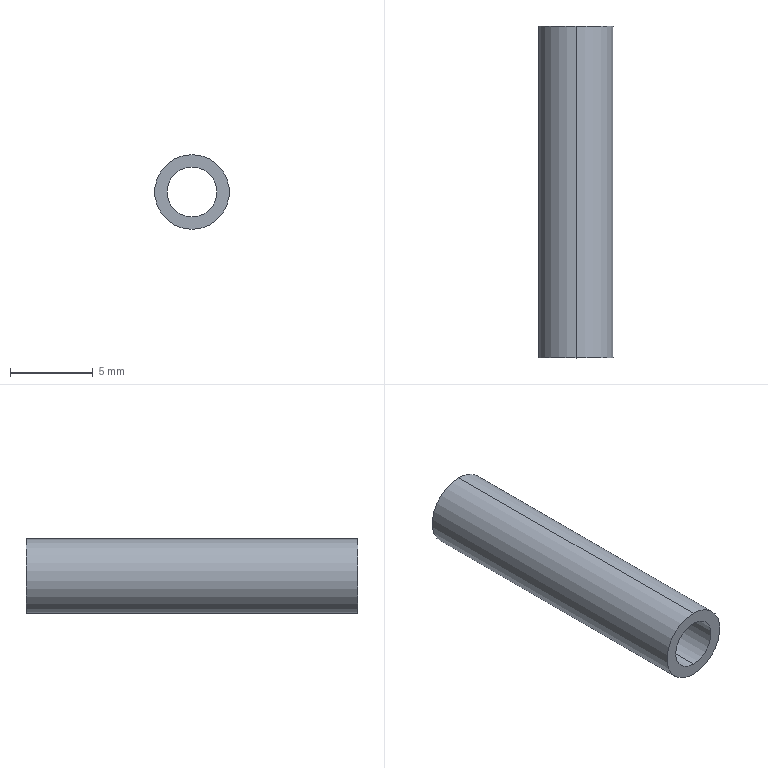Part | SolidWorks | features Extrusion 1 | 1 solid | 6 faces | box 4.5 x 20 x 4.5 mm | volume 176.715 mm3 | cylinder 4 | plane 2 | commonest cylinder face diameters 3 x2 4.5 x2
STEP:
#1=CARTESIAN_POINT('',(0.,20.,-1.5));
#2=VERTEX_POINT('',#1);
#3=CARTESIAN_POINT('',(0.,20.,1.5));
#4=VERTEX_POINT('',#3);
#5=CARTESIAN_POINT('',(0.,20.,0.));
#6=DIRECTION('',(0.,1.,0.));
#7=DIRECTION('',(0.,0.,1.));
#8=AXIS2_PLACEMENT_3D('',#5,#6,#7);
#9=CIRCLE('',#8,1.5);
#10=EDGE_CURVE('',#2,#4,#9,.T.);
#11=ORIENTED_EDGE('',*,*,#10,.T.);
#12=CARTESIAN_POINT('',(0.,0.,1.5));
#13=VERTEX_POINT('',#12);
#14=CARTESIAN_POINT('',(0.,20.,1.5));
#15=DIRECTION('',(0.,-1.,0.));
#16=VECTOR('',#15,1000.);
#17=LINE('',#14,#16);
#18=EDGE_CURVE('',#4,#13,#17,.T.);
#19=ORIENTED_EDGE('',*,*,#18,.T.);
#20=CARTESIAN_POINT('',(0.,0.,-1.5));
#21=VERTEX_POINT('',#20);
#22=CARTESIAN_POINT('',(0.,0.,0.));
#23=DIRECTION('',(0.,1.,0.));
#24=DIRECTION('',(0.,0.,1.));
#25=AXIS2_PLACEMENT_3D('',#22,#23,#24);
#26=CIRCLE('',#25,1.5);
#27=EDGE_CURVE('',#21,#13,#26,.T.);
#28=ORIENTED_EDGE('',*,*,#27,.F.);
#29=CARTESIAN_POINT('',(0.,20.,-1.5));
#30=DIRECTION('',(0.,-1.,0.));
#31=VECTOR('',#30,1000.);
#32=LINE('',#29,#31);
#33=EDGE_CURVE('',#2,#21,#32,.T.);
#34=ORIENTED_EDGE('',*,*,#33,.F.);
#35=EDGE_LOOP('',(#11,#19,#28,#34));
#36=FACE_OUTER_BOUND('',#35,.T.);
#37=CARTESIAN_POINT('',(0.,20.,0.));
#38=DIRECTION('',(0.,-1.,0.));
#39=DIRECTION('',(0.,0.,-1.));
#40=AXIS2_PLACEMENT_3D('',#37,#38,#39);
#41=CYLINDRICAL_SURFACE('',#40,1.5);
#42=ADVANCED_FACE('',(#36),#41,.F.);
#43=CARTESIAN_POINT('',(0.,20.,2.25));
#44=VERTEX_POINT('',#43);
#45=CARTESIAN_POINT('',(0.,20.,-2.25));
#46=VERTEX_POINT('',#45);
#47=CARTESIAN_POINT('',(0.,20.,0.));
#48=DIRECTION('',(0.,1.,0.));
#49=DIRECTION('',(0.,0.,1.));
#50=AXIS2_PLACEMENT_3D('',#47,#48,#49);
#51=CIRCLE('',#50,2.25);
#52=EDGE_CURVE('',#44,#46,#51,.T.);
#53=ORIENTED_EDGE('',*,*,#52,.F.);
#54=CARTESIAN_POINT('',(0.,0.,2.25));
#55=VERTEX_POINT('',#54);
#56=CARTESIAN_POINT('',(0.,20.,2.25));
#57=DIRECTION('',(0.,-1.,0.));
#58=VECTOR('',#57,1000.);
#59=LINE('',#56,#58);
#60=EDGE_CURVE('',#44,#55,#59,.T.);
#61=ORIENTED_EDGE('',*,*,#60,.T.);
#62=CARTESIAN_POINT('',(0.,0.,-2.25));
#63=VERTEX_POINT('',#62);
#64=CARTESIAN_POINT('',(0.,0.,0.));
#65=DIRECTION('',(0.,1.,0.));
#66=DIRECTION('',(0.,0.,1.));
#67=AXIS2_PLACEMENT_3D('',#64,#65,#66);
#68=CIRCLE('',#67,2.25);
#69=EDGE_CURVE('',#55,#63,#68,.T.);
#70=ORIENTED_EDGE('',*,*,#69,.T.);
#71=CARTESIAN_POINT('',(0.,20.,-2.25));
#72=DIRECTION('',(0.,-1.,0.));
#73=VECTOR('',#72,1000.);
#74=LINE('',#71,#73);
#75=EDGE_CURVE('',#46,#63,#74,.T.);
#76=ORIENTED_EDGE('',*,*,#75,.F.);
#77=EDGE_LOOP('',(#53,#61,#70,#76));
#78=FACE_OUTER_BOUND('',#77,.T.);
#79=CARTESIAN_POINT('',(0.,20.,0.));
#80=DIRECTION('',(0.,-1.,0.));
#81=DIRECTION('',(0.,0.,-1.));
#82=AXIS2_PLACEMENT_3D('',#79,#80,#81);
#83=CYLINDRICAL_SURFACE('',#82,2.25);
#84=ADVANCED_FACE('',(#78),#83,.T.);
#85=CARTESIAN_POINT('',(0.,20.,0.));
#86=DIRECTION('',(0.,1.,0.));
#87=DIRECTION('',(0.,0.,1.));
#88=AXIS2_PLACEMENT_3D('',#85,#86,#87);
#89=CIRCLE('',#88,2.25);
#90=EDGE_CURVE('',#46,#44,#89,.T.);
#91=ORIENTED_EDGE('',*,*,#90,.T.);
#92=ORIENTED_EDGE('',*,*,#52,.T.);
#93=EDGE_LOOP('',(#91,#92));
#94=FACE_OUTER_BOUND('',#93,.T.);
#95=ORIENTED_EDGE('',*,*,#10,.F.);
#96=CARTESIAN_POINT('',(0.,20.,0.));
#97=DIRECTION('',(0.,1.,0.));
#98=DIRECTION('',(0.,0.,1.));
#99=AXIS2_PLACEMENT_3D('',#96,#97,#98);
#100=CIRCLE('',#99,1.5);
#101=EDGE_CURVE('',#4,#2,#100,.T.);
#102=ORIENTED_EDGE('',*,*,#101,.F.);
#103=EDGE_LOOP('',(#95,#102));
#104=FACE_BOUND('',#103,.T.);
#105=CARTESIAN_POINT('',(0.,20.,0.));
#106=DIRECTION('',(0.,1.,0.));
#107=DIRECTION('',(0.,0.,1.));
#108=AXIS2_PLACEMENT_3D('',#105,#106,#107);
#109=PLANE('',#108);
#110=ADVANCED_FACE('',(#94,#104),#109,.T.);
#111=CARTESIAN_POINT('',(0.,0.,0.));
#112=DIRECTION('',(0.,1.,0.));
#113=DIRECTION('',(0.,0.,1.));
#114=AXIS2_PLACEMENT_3D('',#111,#112,#113);
#115=CIRCLE('',#114,2.25);
#116=EDGE_CURVE('',#63,#55,#115,.T.);
#117=ORIENTED_EDGE('',*,*,#116,.F.);
#118=ORIENTED_EDGE('',*,*,#69,.F.);
#119=EDGE_LOOP('',(#117,#118));
#120=FACE_OUTER_BOUND('',#119,.T.);
#121=ORIENTED_EDGE('',*,*,#27,.T.);
#122=CARTESIAN_POINT('',(0.,0.,0.));
#123=DIRECTION('',(0.,1.,0.));
#124=DIRECTION('',(0.,0.,1.));
#125=AXIS2_PLACEMENT_3D('',#122,#123,#124);
#126=CIRCLE('',#125,1.5);
#127=EDGE_CURVE('',#13,#21,#126,.T.);
#128=ORIENTED_EDGE('',*,*,#127,.T.);
#129=EDGE_LOOP('',(#121,#128));
#130=FACE_BOUND('',#129,.T.);
#131=CARTESIAN_POINT('',(0.,0.,0.));
#132=DIRECTION('',(0.,1.,0.));
#133=DIRECTION('',(0.,0.,1.));
#134=AXIS2_PLACEMENT_3D('',#131,#132,#133);
#135=PLANE('',#134);
#136=ADVANCED_FACE('',(#120,#130),#135,.F.);
#137=ORIENTED_EDGE('',*,*,#60,.F.);
#138=ORIENTED_EDGE('',*,*,#90,.F.);
#139=ORIENTED_EDGE('',*,*,#75,.T.);
#140=ORIENTED_EDGE('',*,*,#116,.T.);
#141=EDGE_LOOP('',(#137,#138,#139,#140));
#142=FACE_OUTER_BOUND('',#141,.T.);
#143=CARTESIAN_POINT('',(0.,20.,0.));
#144=DIRECTION('',(0.,-1.,0.));
#145=DIRECTION('',(0.,0.,-1.));
#146=AXIS2_PLACEMENT_3D('',#143,#144,#145);
#147=CYLINDRICAL_SURFACE('',#146,2.25);
#148=ADVANCED_FACE('',(#142),#147,.T.);
#149=ORIENTED_EDGE('',*,*,#18,.F.);
#150=ORIENTED_EDGE('',*,*,#101,.T.);
#151=ORIENTED_EDGE('',*,*,#33,.T.);
#152=ORIENTED_EDGE('',*,*,#127,.F.);
#153=EDGE_LOOP('',(#149,#150,#151,#152));
#154=FACE_OUTER_BOUND('',#153,.T.);
#155=CARTESIAN_POINT('',(0.,20.,0.));
#156=DIRECTION('',(0.,-1.,0.));
#157=DIRECTION('',(0.,0.,-1.));
#158=AXIS2_PLACEMENT_3D('',#155,#156,#157);
#159=CYLINDRICAL_SURFACE('',#158,1.5);
#160=ADVANCED_FACE('',(#154),#159,.F.);
#161=CLOSED_SHELL('',(#42,#84,#110,#136,#148,#160));
#162=MANIFOLD_SOLID_BREP('',#161);
#163=CARTESIAN_POINT('',(0.,0.,0.));
#164=DIRECTION('',(0.,0.,1.));
#165=DIRECTION('',(1.,0.,0.));
#166=AXIS2_PLACEMENT_3D('',#163,#164,#165);
#167=(LENGTH_UNIT()NAMED_UNIT(*)SI_UNIT(.MILLI.,.METRE.));
#168=UNCERTAINTY_MEASURE_WITH_UNIT(LENGTH_MEASURE(0.00001),#167,'','');
#169=(NAMED_UNIT(*)PLANE_ANGLE_UNIT()SI_UNIT($,.RADIAN.));
#170=(NAMED_UNIT(*)SI_UNIT($,.STERADIAN.)SOLID_ANGLE_UNIT());
#171=(GEOMETRIC_REPRESENTATION_CONTEXT(3)GLOBAL_UNCERTAINTY_ASSIGNED_CONTEXT((#168))GLOBAL_UNIT_ASSIGNED_CONTEXT((#167,#169,#170))REPRESENTATION_CONTEXT('',''));
#172=ADVANCED_BREP_SHAPE_REPRESENTATION('',(#162,#166),#171);